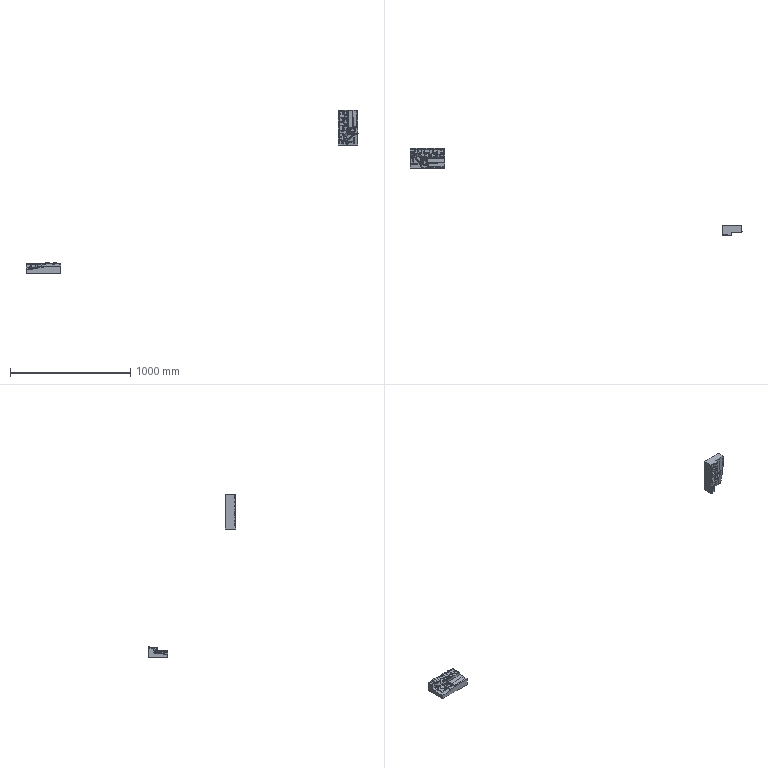NC program | NX | posted with a generic post | part box 2756 x 729.572 x 1353 mm
Lines 37177 to 38047 of 180527:
(STREAMLINE , TOOL : B6)
N74334 M6
N74336 G54
N74338 G17 G0 G90 X286.496 Y153.625 B0. C0. S3000 M3
N74340 G43 Z10. H0
N74342 Z-2.
N74344 G94 G1 Z-7.768 F2500.
N74346 X281.919
N74348 X279.629 Z-7.759
N74350 X277.339 Z-7.719
N74352 X268.2 Y153.624 Z-7.574
N74354 X265.889 Y153.623 Z-7.541
N74356 X263.472 Z-7.507
N74358 X262.453 Z-7.486
N74360 X261.884 Z-7.423
N74362 X261.325 Y153.622 Z-7.305
N74364 X260.778 Z-7.133
N74366 X260.25 Y153.621 Z-6.911
N74368 X259.746 Y153.62 Z-6.64
N74370 X259.271 Y153.619 Z-6.322
N74372 X258.828 Y153.618 Z-5.96
N74374 X258.416 Y153.617 Z-5.561
N74376 X258.01 Y153.616 Z-5.158
N74378 X257.578 Y153.615 Z-4.781
N74380 X257.114 Y153.614 Z-4.448
N74382 X256.619 Y153.613 Z-4.16
N74384 X256.098 Y153.612 Z-3.921
N74386 X255.558 Z-3.732
N74388 X255.002 Y153.611 Z-3.595
N74390 X254.438 Z-3.514
N74392 X253.292 Z-3.475
N74394 X251.002 Y153.61 Z-3.437
N74396 X241.841 Y153.609 Z-3.298
N74398 X232.68 Y153.608 Z-3.182
N74400 X230.389 Z-3.156
N74402 X228.099 Z-3.144
N74404 X227.53 Z-3.201
N74406 X226.969 Z-3.313
N74408 X226.42 Y153.609 Z-3.478
N74410 X225.89 Z-3.694
N74412 X225.382 Y153.61 Z-3.959
N74414 X224.904 Y153.611 Z-4.271
N74416 X224.458 Y153.612 Z-4.627
N74418 X224.041 Y153.613 Z-5.023
N74420 X223.21 Y153.615 Z-5.811
N74422 X222.756 Y153.616 Z-6.159
N74424 X222.271 Y153.617 Z-6.461
N74426 X221.756 Y153.618 Z-6.716
N74428 X221.222 Z-6.92
N74430 X220.671 Y153.619 Z-7.073
N74432 X220.107 Z-7.173
N74434 X219.537 Z-7.218
N74436 X218.964 Z-7.221
N74438 X217.847
N74440 X215.489 Z-7.225
N74442 X206.373 Y153.618 Z-7.252
N74444 X203.936 Z-7.261
N74446 X201.559 Z-7.271
N74448 X199.489 Z-7.282
N74450 X198.923 Z-7.285
N74452 X198.35 Z-7.266
N74454 X197.783 Y153.617 Z-7.192
N74456 X197.226 Z-7.063
N74458 X196.682 Y153.616 Z-6.881
N74460 X196.159 Z-6.65
N74462 X195.66 Y153.615 Z-6.369
N74464 X195.191 Y153.614 Z-6.042
N74466 X194.755 Y153.613 Z-5.672
N74468 X194.345 Y153.612 Z-5.27
N74470 X193.922 Y153.611 Z-4.886
N74472 X193.471 Y153.609 Z-4.532
N74474 X192.997 Y153.608 Z-4.212
N74476 X192.501 Z-3.927
N74478 X191.985 Y153.607 Z-3.678
N74480 X191.453 Y153.606 Z-3.466
N74482 X190.907 Z-3.293
N74484 X190.351 Y153.605 Z-3.16
N74486 X189.786 Z-3.066
N74488 X189.216 Z-3.013
N74490 X188.644 Z-3.001
N74492 X188.071 Z-3.011
N74494 X186.926 Z-3.032
N74496 X184.636 Z-3.074
N74498 X182.346 Z-3.118
N74500 X180.056 Z-3.163
N74502 X170.896 Y153.604 Z-3.361
N74504 X168.606 Z-3.414
N74506 X166.317 Z-3.469
N74508 X164.027 Z-3.526
N74510 X163.454 Z-3.545
N74512 X162.884 Y153.605 Z-3.598
N74514 X162.32 Z-3.693
N74516 X161.763 Z-3.827
N74518 X161.218 Y153.606 Z-4.002
N74520 X160.687 Z-4.215
N74522 X160.172 Y153.607 Z-4.464
N74524 X159.676 Y153.608 Z-4.751
N74526 X159.202 Y153.609 Z-5.072
N74528 X158.752 Y153.61 Z-5.426
N74530 X157.915 Y153.612 Z-6.207
N74532 X157.466 Y153.613 Z-6.563
N74534 X156.987 Y153.614 Z-6.873
N74536 X156.477 Z-7.138
N74538 X155.947 Y153.615 Z-7.352
N74540 X155.398 Z-7.516
N74542 X154.837 Y153.616 Z-7.626
N74544 X154.268 Z-7.681
N74546 X153.695 Z-7.691
N74548 X144.534 Y153.615 Z-7.737
N74550 X133.081 Z-7.773
N74552 X126.21 Y153.614 Z-7.781
N74554 X123.849 Z-7.782
N74556 X121.629
N74558 X121.342 Z-7.777
N74560 X121.058 Z-7.747
N74562 X120.778 Y153.613 Z-7.69
N74564 X120.504 Z-7.606
N74566 X120.24 Z-7.496
N74568 X119.987 Y153.612 Z-7.362
N74570 X119.497 Y153.611 Z-7.065
N74572 X118.999 Z-6.789
N74574 X118.485 Y153.61 Z-6.529
N74576 X117.966 Y153.609 Z-6.29
N74578 X117.437 Y153.608 Z-6.07
N74580 X116.9 Z-5.871
N74582 X116.356 Y153.607 Z-5.692
N74584 X115.806 Z-5.534
N74586 X115.249 Y153.606 Z-5.399
N74588 X114.683 Z-5.32
N74590 X114.11 Z-5.307
N74592 X112.966 Z-5.347
N74594 X108.388 Z-5.507
N74596 X99.231 Z-5.828
N74598 X96.942 Y153.607 Z-5.908
N74600 X95.798 Z-5.948
N74602 X95.225 Z-5.969
N74604 X94.656 Z-6.027
N74606 X94.098 Z-6.151
N74608 X93.557 Y153.608 Z-6.337
N74610 X92.53 Y153.609 Z-6.86
N74612 X91.543 Y153.611 Z-7.425
N74614 X90.999 Z-7.602
N74616 X90.433 Z-7.673
N74618 X81.268 Y153.61 Z-7.606
N74620 X72.108 Y153.609 Z-7.519
N74622 X70.964 Z-7.507
N74624 X70.397 Z-7.436
N74626 X69.853 Y153.608 Z-7.258
N74628 X67.878 Y153.605 Z-6.103
N74630 X66.843 Y153.603 Z-5.612
N74632 X65.775 Y153.602 Z-5.202
N74634 X64.677 Y153.601 Z-4.873
N74636 X63.559 Y153.6 Z-4.628
N74638 X62.425 Z-4.47
N74640 X61.282 Z-4.4
N74642 X47.54 Y153.598 Z-4.241
N74644 X46.395 Z-4.263
N74646 X45.256 Z-4.373
N74648 X44.132 Y153.599 Z-4.57
N74650 X43.018 Y153.6 Z-4.854
N74652 X41.934 Y153.601 Z-5.219
N74654 X40.88 Y153.602 Z-5.666
N74656 X39.861 Y153.603 Z-6.19
N74658 X38.879 Y153.605 Z-6.78
N74660 X38.351 Z-6.997
N74662 X37.79 Y153.606 Z-7.109
N74664 X36.645 Z-7.116
N74666 X0. Y153.605 Z-6.692
N74668 Z-6.832
N74670 X36.661 Y153.606 Z-7.256
N74672 X37.807 Z-7.25
N74674 X38.369 Y153.605 Z-7.14
N74676 X38.898 Z-6.925
N74678 X39.879 Y153.603 Z-6.334
N74680 X40.892 Y153.602 Z-5.8
N74682 X41.943 Y153.601 Z-5.347
N74684 X43.027 Y153.6 Z-4.979
N74686 X44.141 Y153.599 Z-4.697
N74688 X45.267 Y153.598 Z-4.506
N74690 X46.406 Z-4.401
N74692 X47.552 Z-4.381
N74694 X61.3 Y153.6 Z-4.54
N74696 X62.444 Z-4.608
N74698 X63.579 Z-4.762
N74700 X64.697 Y153.601 Z-5.007
N74702 X65.794 Y153.602 Z-5.341
N74704 X66.858 Y153.604 Z-5.759
N74706 X67.887 Y153.605 Z-6.261
N74708 X69.864 Y153.608 Z-7.408
N74710 X70.41 Y153.609 Z-7.579
N74712 X70.977 Z-7.647
N74714 X72.122 Z-7.659
N74716 X83.562 Y153.611 Z-7.764
N74718 X90.455 Z-7.813
N74720 X91.022 Z-7.745
N74722 X91.567 Y153.61 Z-7.571
N74724 X92.552 Y153.609 Z-7.003
N74726 X93.578 Y153.607 Z-6.478
N74728 X94.118 Z-6.289
N74730 X94.676 Z-6.163
N74732 X95.245 Z-6.1
N74734 X95.817 Z-6.076
N74736 X96.962 Z-6.035
N74738 X99.252 Y153.606 Z-5.954
N74740 X108.412 Z-5.633
N74742 X112.992 Z-5.473
N74744 X114.137 Z-5.436
N74746 X114.71 Z-5.454
N74748 X115.276 Z-5.535
N74750 X115.832 Y153.607 Z-5.672
N74752 X116.382 Z-5.833
N74754 X116.924 Y153.608 Z-6.016
N74756 X117.458 Z-6.221
N74758 X117.985 Y153.609 Z-6.446
N74760 X118.499 Y153.61 Z-6.691
N74762 X119.51 Y153.612 Z-7.232
N74764 X120.003 Z-7.52
N74766 X120.257 Y153.613 Z-7.648
N74768 X120.522 Z-7.753
N74770 X120.798 Z-7.833
N74772 X121.078 Y153.614 Z-7.888
N74774 X121.362 Z-7.917
N74776 X121.648 Z-7.922
N74778 X123.873 Z-7.921
N74780 X126.232
N74782 X137.689 Y153.615 Z-7.902
N74784 X144.564 Z-7.877
N74786 X153.729 Y153.616 Z-7.83
N74788 X154.303 Z-7.821
N74790 X154.872 Z-7.768
N74792 X155.434 Y153.615 Z-7.662
N74794 X155.984 Z-7.506
N74796 X156.516 Y153.614 Z-7.3
N74798 X157.029 Z-7.047
N74800 X157.512 Y153.613 Z-6.746
N74802 X157.963 Y153.612 Z-6.394
N74804 X158.797 Y153.609 Z-5.61
N74806 X159.243 Y153.608 Z-5.251
N74808 X159.713 Z-4.925
N74810 X160.205 Y153.607 Z-4.634
N74812 X160.717 Y153.606 Z-4.379
N74814 X161.246 Z-4.161
N74816 X161.79 Y153.605 Z-3.982
N74818 X162.345 Z-3.843
N74820 X162.908 Z-3.744
N74822 X163.478 Y153.604 Z-3.686
N74824 X164.05 Z-3.663
N74826 X166.341 Z-3.604
N74828 X168.631 Z-3.549
N74830 X170.922 Z-3.496
N74832 X180.086 Y153.605 Z-3.298
N74834 X182.377 Z-3.252
N74836 X184.668 Z-3.209
N74838 X186.959 Z-3.167
N74840 X188.104 Z-3.154
N74842 X188.676 Z-3.151
N74844 X189.247 Z-3.17
N74846 X189.816 Z-3.231
N74848 X190.378 Z-3.333
N74850 X190.931 Y153.606 Z-3.474
N74852 X191.473 Z-3.655
N74854 X192. Y153.607 Z-3.875
N74856 X192.51 Y153.608 Z-4.131
N74858 X193. Z-4.424
N74860 X193.468 Y153.609 Z-4.751
N74862 X195.199 Y153.614 Z-6.236
N74864 X195.673 Y153.615 Z-6.549
N74866 X196.176 Y153.616 Z-6.817
N74868 X196.701 Y153.617 Z-7.039
N74870 X197.247 Z-7.213
N74872 X197.805 Z-7.336
N74874 X198.372 Y153.618 Z-7.406
N74876 X198.945 Z-7.425
N74878 X199.511 Z-7.422
N74880 X201.592 Z-7.411
N74882 X203.966 Z-7.4
N74884 X206.398 Z-7.391
N74886 X215.521 Y153.619 Z-7.365
N74888 X217.877 Z-7.361
N74890 X218.995
N74892 X219.568 Z-7.358
N74894 X220.139 Z-7.315
N74896 X220.703 Z-7.22
N74898 X221.256 Y153.618 Z-7.073
N74900 X221.792 Z-6.877
N74902 X222.309 Y153.617 Z-6.633
N74904 X222.798 Y153.616 Z-6.341
N74906 X223.255 Y153.615 Z-5.999
N74908 X223.677 Y153.614 Z-5.611
N74910 X224.083 Y153.613 Z-5.208
N74912 X224.495 Y153.612 Z-4.808
N74914 X224.937 Y153.611 Z-4.446
N74916 X225.41 Y153.61 Z-4.129
N74918 X225.914 Y153.609 Z-3.858
N74920 X226.44 Z-3.635
N74922 X226.986 Y153.608 Z-3.463
N74924 X227.544 Z-3.344
N74926 X228.111 Z-3.278
N74928 X230.399 Z-3.266
N74930 X232.69 Z-3.289
N74932 X241.856 Y153.609 Z-3.399
N74934 X251.02 Y153.61 Z-3.532
N74936 X253.309 Y153.611 Z-3.589
N74938 X254.45 Z-3.648
N74940 X255.012 Z-3.74
N74942 X255.563 Y153.612 Z-3.885
N74944 X256.098 Z-4.083
N74946 X256.614 Y153.613 Z-4.331
N74948 X257.103 Y153.614 Z-4.625
N74950 X257.561 Y153.615 Z-4.965
N74952 X257.985 Y153.616 Z-5.347
N74954 X258.388 Y153.617 Z-5.754
N74956 X258.802 Y153.618 Z-6.151
N74958 X259.248 Y153.619 Z-6.507
N74960 X259.727 Y153.62 Z-6.814
N74962 X260.235 Y153.621 Z-7.074
N74964 X260.764 Y153.622 Z-7.287
N74966 X261.313 Z-7.452
N74968 X261.873 Y153.623 Z-7.565
N74970 X262.442 Z-7.626
N74972 X263.467 Z-7.647
N74974 X265.879 Z-7.681
N74976 X268.191 Y153.624 Z-7.714
N74978 X277.335 Y153.625 Z-7.859
N74980 X279.626 Z-7.899
N74982 X281.917 Z-7.907
N74984 X286.496
N74986 Z-8.047
N74988 X281.915
N74990 X279.623 Z-8.039
N74992 X277.331 Z-7.999
N74994 X268.182 Y153.624 Z-7.854
N74996 X265.87 Y153.623 Z-7.82
N74998 X263.463 Z-7.787
N75000 X262.432 Z-7.766
N75002 X261.862 Z-7.708
N75004 X261.301 Y153.622 Z-7.599
N75006 X260.751 Z-7.441
N75008 X260.219 Y153.621 Z-7.237
N75010 X259.709 Y153.62 Z-6.989
N75012 X259.225 Y153.619 Z-6.692
N75014 X258.775 Y153.618 Z-6.342
N75016 X258.36 Y153.617 Z-5.946
N75018 X257.961 Y153.616 Z-5.536
N75020 X257.543 Y153.615 Z-5.148
N75022 X257.091 Y153.614 Z-4.802
N75024 X256.608 Y153.613 Z-4.501
N75026 X256.098 Y153.612 Z-4.245
N75028 X255.568 Z-4.039
N75030 X255.021 Y153.611 Z-3.884
N75032 X254.463 Z-3.782
N75034 X253.895 Z-3.732
N75036 X253.326 Z-3.703
N75038 X251.039 Y153.61 Z-3.628
N75040 X241.87 Y153.609 Z-3.5
N75042 X232.701 Y153.608 Z-3.396
N75044 X230.409 Z-3.375
N75046 X229.264 Z-3.38
N75048 X228.123 Z-3.412
N75050 X227.558 Z-3.486
N75052 X227.003 Z-3.613
N75054 X226.46 Y153.609 Z-3.793
N75056 X225.938 Z-4.022
N75058 X225.438 Y153.61 Z-4.3
N75060 X224.969 Y153.611 Z-4.622
N75062 X224.532 Y153.612 Z-4.988
N75064 X224.126 Y153.613 Z-5.393
N75066 X223.723 Y153.614 Z-5.799
N75068 X223.301 Y153.615 Z-6.186
N75070 X222.839 Y153.616 Z-6.524
N75072 X222.347 Y153.617 Z-6.805
N75074 X221.827 Y153.618 Z-7.038
N75076 X221.289 Z-7.226
N75078 X220.735 Y153.619 Z-7.366
N75080 X220.171 Z-7.457
N75082 X219.6 Z-7.498
N75084 X219.026 Z-7.5
N75086 X217.906 Z-7.501
N75088 X215.552 Z-7.505
N75090 X206.424 Y153.618 Z-7.531
N75092 X203.997 Z-7.54
N75094 X201.626 Z-7.55
N75096 X199.534 Z-7.561
N75098 X198.967 Z-7.565
N75100 X198.394 Z-7.547
N75102 X197.826 Y153.617 Z-7.48
N75104 X197.268 Z-7.363
N75106 X196.72 Z-7.196
N75108 X196.193 Y153.616 Z-6.985
N75110 X195.687 Y153.615 Z-6.728
N75112 X195.208 Y153.614 Z-6.43
N75114 X193.465 Y153.609 Z-4.971
N75116 X193.004 Z-4.637
N75118 X192.52 Y153.608 Z-4.336
N75120 X192.015 Y153.607 Z-4.072
N75122 X191.493 Y153.606 Z-3.844
N75124 X190.955 Z-3.655
N75126 X190.405 Y153.605 Z-3.506
N75128 X189.845 Z-3.396
N75130 X189.279 Z-3.328
N75132 X188.709 Z-3.301
N75134 X188.137 Z-3.297
N75136 X186.993 Z-3.302
N75138 X184.7 Z-3.343
N75140 X182.408 Z-3.387
N75142 X180.116 Z-3.433
N75144 X170.948 Y153.604 Z-3.63
N75146 X168.656 Z-3.684
N75148 X166.365 Z-3.739
N75150 X164.073 Z-3.8
N75152 X163.501 Z-3.827
N75154 X162.932 Y153.605 Z-3.889
N75156 X162.37 Z-3.993
N75158 X161.816 Z-4.137
N75160 X161.275 Y153.606 Z-4.321
N75162 X160.748 Z-4.544
N75164 X160.239 Y153.607 Z-4.804
N75166 X159.75 Y153.608 Z-5.1
N75168 X159.284 Z-5.431
N75170 X158.843 Y153.609 Z-5.795
N75172 X158.012 Y153.612 Z-6.582
N75174 X157.558 Y153.613 Z-6.929
N75176 X157.071 Z-7.22
N75178 X156.555 Y153.614 Z-7.462
N75180 X156.021 Y153.615 Z-7.659
N75182 X155.47 Z-7.809
N75184 X154.907 Y153.616 Z-7.91
N75186 X154.337 Z-7.961
N75188 X153.763 Z-7.97
N75190 X144.594 Y153.615 Z-8.017
N75192 X133.131 Z-8.052
N75194 X126.254 Y153.614 Z-8.06
N75196 X123.897 Z-8.061
N75198 X121.668 Z-8.062
N75200 X121.382 Z-8.057
N75202 X121.097 Z-8.029
N75204 X120.817 Y153.613 Z-7.977
N75206 X120.541 Z-7.9
N75208 X120.274 Z-7.8
N75210 X120.019 Y153.612 Z-7.677
N75212 X119.522 Z-7.398
N75214 X118.514 Y153.61 Z-6.854
N75216 X118.003 Y153.609 Z-6.603
N75218 X117.48 Z-6.371
N75220 X116.948 Y153.608 Z-6.162
N75222 X116.407 Y153.607 Z-5.975
N75224 X115.858 Z-5.811
N75226 X115.303 Y153.606 Z-5.671
N75228 X114.737 Z-5.587
N75230 X114.165 Z-5.566
N75232 X113.019 Z-5.599
N75234 X108.437 Z-5.76
N75236 X99.273 Z-6.081
N75238 X96.982 Y153.607 Z-6.161
N75240 X95.836 Z-6.204
N75242 X95.264 Z-6.231
N75244 X94.696 Z-6.298
N75246 X94.139 Z-6.427
N75248 X93.599 Z-6.618
N75250 X93.082 Y153.608 Z-6.866
N75252 X92.575 Y153.609 Z-7.147
N75254 X92.09 Y153.61 Z-7.444
N75256 X91.847 Z-7.592
N75258 X91.59 Z-7.717
N75260 X91.322 Y153.611 Z-7.816
N75262 X91.044 Z-7.888
N75264 X90.762 Z-7.933
N75266 X90.477 Z-7.953
N75268 X81.304 Y153.61 Z-7.885
N75270 X72.136 Y153.609 Z-7.799
N75272 X70.99 Z-7.787
N75274 X70.423 Z-7.722
N75276 X69.875 Z-7.558
N75278 X67.895 Y153.605 Z-6.419
N75280 X66.873 Y153.604 Z-5.906
N75282 X65.812 Y153.602 Z-5.479
N75284 X64.717 Y153.601 Z-5.141
N75286 X63.598 Y153.6 Z-4.895
N75288 X62.463 Z-4.745
N75290 X61.318 Z-4.68
N75292 X47.564 Y153.598 Z-4.521
N75294 X46.418 Z-4.54
N75296 X45.278 Z-4.639
N75298 X44.15 Y153.599 Z-4.824
N75300 X43.036 Y153.6 Z-5.105
N75302 X41.952 Y153.601 Z-5.475
N75304 X40.904 Y153.602 Z-5.934
N75306 X38.916 Y153.605 Z-7.071
N75308 X38.386 Z-7.283
N75310 X37.824 Y153.606 Z-7.391
N75312 X36.678 Z-7.396
N75314 X0. Y153.605 Z-6.972
N75316 Z-7.112
N75318 X36.694 Y153.606 Z-7.535
N75320 X37.841 Z-7.532
N75322 X38.403 Y153.605 Z-7.426
N75324 X38.935 Z-7.216
N75326 X40.916 Y153.602 Z-6.069
N75328 X41.961 Y153.601 Z-5.603
N75330 X43.045 Y153.6 Z-5.23
N75332 X44.16 Y153.599 Z-4.951
N75334 X45.289 Y153.598 Z-4.772
N75336 X46.429 Z-4.678
N75338 X47.576 Z-4.66
N75340 X61.337 Y153.6 Z-4.82
N75342 X62.481 Z-4.883
N75344 X63.618 Z-5.029
N75346 X64.737 Y153.601 Z-5.275
N75348 X65.831 Y153.602 Z-5.618
N75350 X66.889 Y153.604 Z-6.053
N75352 X67.903 Y153.605 Z-6.578
N75354 X69.887 Y153.609 Z-7.708
N75356 X70.436 Z-7.864
N75358 X71.004 Z-7.927
N75360 X72.15 Z-7.939
N75362 X83.602 Y153.611 Z-8.044
N75364 X90.499 Z-8.093
N75366 X90.784 Z-8.074
N75368 X91.067 Z-8.031
N75370 X91.345 Z-7.961
N75372 X91.614 Y153.61 Z-7.863
N75374 X91.871 Z-7.739
N75376 X92.114 Z-7.591
N75378 X92.598 Y153.609 Z-7.291
N75380 X93.104 Y153.608 Z-7.008
N75382 X93.62 Y153.607 Z-6.758
N75384 X94.159 Z-6.565
N75386 X94.715 Z-6.433
N75388 X95.284 Z-6.363
N75390 X95.855 Z-6.332
N75392 X97.001 Z-6.288
N75394 X99.293 Y153.606 Z-6.207
N75396 X108.462 Z-5.886
N75398 X110.754 Z-5.805
N75400 X113.046 Z-5.725
N75402 X114.192 Z-5.696
N75404 X114.764 Z-5.72
N75406 X115.329 Z-5.808
N75408 X115.885 Y153.607 Z-5.949
N75410 X116.433 Z-6.117
N75412 X116.972 Y153.608 Z-6.308
N75414 X117.502 Y153.609 Z-6.522
N75416 X118.022 Z-6.759
N75418 X118.529 Y153.61 Z-7.017
N75420 X119.535 Y153.612 Z-7.565
N75422 X120.034 Z-7.835
N75424 X120.292 Y153.613 Z-7.952
N75426 X120.559 Z-8.047
N75428 X120.836 Z-8.121
N75430 X121.117 Y153.614 Z-8.17
N75432 X121.402 Z-8.197
N75434 X121.688 Z-8.201
N75436 X123.921
N75438 X126.276 Z-8.2
N75440 X137.743 Y153.615 Z-8.181
N75442 X144.624 Z-8.156
N75444 X153.798 Y153.616 Z-8.109
N75446 X154.372 Z-8.101
N75448 X154.942 Z-8.052
N75450 X155.505 Y153.615 Z-7.955
N75452 X156.058 Z-7.812
N75454 X156.594 Y153.614 Z-7.624
N75456 X157.112 Y153.613 Z-7.393
N75458 X157.603 Y153.612 Z-7.111
N75460 X158.061 Y153.611 Z-6.769
N75462 X158.889 Y153.609 Z-5.979
N75464 X159.325 Y153.608 Z-5.611
N75466 X159.787 Y153.607 Z-5.275
N75468 X160.272 Z-4.974
N75470 X160.779 Y153.606 Z-4.709
N75472 X161.303 Z-4.481
N75474 X161.842 Y153.605 Z-4.292
N75476 X162.395 Z-4.144
N75478 X162.956 Z-4.035
N75480 X163.525 Y153.604 Z-3.968
N75482 X164.096 Z-3.937
N75484 X166.389 Z-3.873
N75486 X168.681 Z-3.818
N75488 X170.974 Z-3.765
N75490 X180.146 Y153.605 Z-3.567
N75492 X182.439 Z-3.522
N75494 X184.732 Z-3.478
N75496 X187.026 Z-3.438
N75498 X188.17 Z-3.44
N75500 X188.741 Z-3.45
N75502 X189.31 Z-3.485
N75504 X189.875 Z-3.561
N75506 X190.432 Z-3.679
N75508 X190.979 Y153.606 Z-3.836
N75510 X191.513 Z-4.033
N75512 X192.031 Y153.607 Z-4.269
N75514 X192.53 Y153.608 Z-4.541
N75516 X193.007 Y153.609 Z-4.849
N75518 X193.462 Z-5.19
N75520 X194.335 Y153.612 Z-5.928
N75522 X194.763 Y153.613 Z-6.298
N75524 X195.217 Y153.614 Z-6.623
N75526 X195.7 Y153.615 Z-6.908
N75528 X196.209 Y153.616 Z-7.152
N75530 X196.739 Y153.617 Z-7.354
N75532 X197.288 Z-7.512
N75534 X197.848 Y153.618 Z-7.624
N75536 X198.416 Z-7.688
N75538 X198.99 Z-7.705
N75540 X199.557 Z-7.701
N75542 X201.659 Z-7.69
N75544 X204.027 Z-7.68
N75546 X206.449 Z-7.671
N75548 X215.583 Y153.619 Z-7.645
N75550 X217.936 Z-7.641
N75552 X220.202 Z-7.599
N75554 X221.323 Y153.618 Z-7.378
N75556 X222.385 Y153.617 Z-6.977
N75558 X222.881 Y153.616 Z-6.706
N75560 X223.346 Y153.615 Z-6.373
N75562 X224.168 Y153.613 Z-5.577
N75564 X225.002 Y153.611 Z-4.798
N75566 X225.962 Y153.609 Z-4.186
N75568 X227.02 Y153.608 Z-3.763
N75570 X228.135 Z-3.546
N75572 X230.418 Z-3.485
N75574 X232.712 Z-3.503
N75576 X241.885 Y153.609 Z-3.601
N75578 X251.058 Y153.61 Z-3.723
N75580 X252.203 Y153.611 Z-3.758
N75582 X253.344 Z-3.818
N75584 X253.911 Z-3.856
N75586 X254.475 Z-3.916
N75588 X255.03 Z-4.028
N75590 X255.573 Y153.612 Z-4.192
N75592 X256.099 Z-4.408
N75594 X256.603 Y153.613 Z-4.671
N75596 X257.08 Y153.614 Z-4.979
N75598 X257.525 Y153.615 Z-5.332
N75600 X257.937 Y153.616 Z-5.726
N75602 X258.332 Y153.617 Z-6.138
N75604 X258.749 Y153.618 Z-6.533
N75606 X259.202 Y153.619 Z-6.877
N75608 X259.69 Y153.62 Z-7.163
N75610 X260.204 Y153.621 Z-7.401
N75612 X260.738 Y153.622 Z-7.595
N75614 X261.289 Z-7.746
N75616 X261.85 Y153.623 Z-7.85
N75618 X262.421 Z-7.906
N75620 X263.458 Z-7.927
N75622 X265.861 Z-7.96
N75624 X268.173 Y153.624 Z-7.993
N75626 X277.326 Y153.625 Z-8.138
N75628 X279.62 Z-8.178
N75630 X281.913 Z-8.187
N75632 X286.496
N75634 Z-8.326
N75636 X281.911
N75638 X279.617 Z-8.318
N75640 X277.322 Z-8.278
N75642 X268.163 Y153.624 Z-8.133
N75644 X265.852 Y153.623 Z-8.1
N75646 X263.453 Z-8.067
N75648 X262.41 Z-8.047
N75650 X261.839 Z-7.993
N75652 X261.277 Y153.622 Z-7.894
N75654 X260.725 Z-7.75
N75656 X260.189 Y153.621 Z-7.564
N75658 X259.672 Y153.62 Z-7.337
N75660 X259.18 Y153.619 Z-7.063
N75662 X258.722 Y153.618 Z-6.724
N75664 X258.305 Y153.617 Z-6.331
N75666 X257.912 Y153.616 Z-5.915
N75668 X257.507 Y153.615 Z-5.516
N75670 X257.068 Y153.614 Z-5.157
N75672 X256.597 Y153.613 Z-4.841
N75674 X256.099 Y153.612 Z-4.57
N75676 X255.578 Z-4.346
N75678 X255.039 Y153.611 Z-4.172
N75680 X254.488 Z-4.05
N75682 X253.926 Z-3.979
N75684 X253.361 Z-3.932
N75686 X252.222 Z-3.859
N75688 X251.077 Y153.61 Z-3.819
N75690 X241.9 Y153.609 Z-3.703
N75692 X232.722 Y153.608 Z-3.61
N75694 X230.428 Z-3.594
N75696 X229.284 Z-3.616
N75698 X228.147 Z-3.68
N75700 X227.586 Z-3.771
N75702 X227.036 Z-3.913
N75704 X226.501 Y153.609 Z-4.107
N75706 X225.986 Z-4.35
N75708 X225.494 Y153.61 Z-4.64
N75710 X225.034 Y153.611 Z-4.973
N75712 X224.607 Y153.612 Z-5.349
N75714 X224.21 Y153.613 Z-5.762
N75716 X223.815 Y153.614 Z-6.176
N75718 X223.391 Y153.615 Z-6.561
N75720 X222.923 Y153.616 Z-6.888
N75722 X222.423 Y153.617 Z-7.15
N75724 X221.898 Y153.618 Z-7.361
N75726 X221.356 Z-7.531
N75728 X220.8 Y153.619 Z-7.658
N75730 X220.234 Z-7.741
N75732 X219.662 Z-7.778
N75734 X219.089 Z-7.78
N75736 X217.965 Z-7.781
N75738 X215.614 Z-7.784
N75740 X206.474 Y153.618 Z-7.81
N75742 X204.058 Z-7.819
N75744 X201.692 Z-7.83
N75746 X199.58 Z-7.841
N75748 X198.438 Z-7.829
N75750 X197.869 Z-7.768
N75752 X197.309 Y153.617 Z-7.662
N75754 X196.758 Z-7.511
N75756 X196.226 Y153.616 Z-7.32
N75758 X195.713 Y153.615 Z-7.087
N75760 X195.226 Y153.614 Z-6.817
N75762 X194.766 Y153.613 Z-6.507
N75764 X194.331 Y153.612 Z-6.147
N75766 X193.458 Y153.609 Z-5.409
N75768 X193.011 Z-5.061
N75770 X192.539 Y153.608 Z-4.745
N75772 X192.046 Y153.607 Z-4.466
N75774 X191.533 Y153.606 Z-4.223
N75776 X191.003 Z-4.018
N75778 X190.459 Y153.605 Z-3.852
N75780 X189.904 Z-3.727
N75782 X189.342 Z-3.642
N75784 X188.774 Z-3.6
N75786 X188.204 Z-3.583
N75788 X187.059 Z-3.573
N75790 X184.765 Z-3.613
N75792 X182.471 Z-3.657
N75794 X180.176 Z-3.702
N75796 X171. Y153.604 Z-3.9
N75798 X168.707 Z-3.953
N75800 X166.413 Z-4.008
N75802 X164.119 Z-4.074
N75804 X163.548 Z-4.109
N75806 X162.98 Y153.605 Z-4.18
N75808 X162.42 Z-4.294
N75810 X161.869 Z-4.447
N75812 X161.331 Z-4.641
N75814 X160.809 Y153.606 Z-4.873
N75816 X160.306 Y153.607 Z-5.143
N75818 X159.823 Z-5.45
N75820 X159.366 Y153.608 Z-5.79
N75822 X158.934 Y153.609 Z-6.163
N75824 X158.11 Y153.611 Z-6.957
N75826 X157.649 Y153.612 Z-7.294
N75828 X157.154 Y153.613 Z-7.566
N75830 X156.633 Y153.614 Z-7.786
N75832 X156.095 Y153.615 Z-7.965
N75834 X155.541 Z-8.102
N75836 X154.977 Y153.616 Z-8.194
N75838 X154.406 Z-8.24
N75840 X153.832 Z-8.249
N75842 X144.654 Y153.615 Z-8.296
N75844 X133.181 Z-8.332
N75846 X126.298 Y153.614 Z-8.34
N75848 X123.945 Z-8.341
N75850 X121.708
N75852 X121.422 Z-8.337
N75854 X121.137 Z-8.312
N75856 X120.855 Y153.613 Z-8.264
N75858 X120.578 Z-8.194
N75860 X120.309 Z-8.104
N75862 X120.05 Y153.612 Z-7.992
N75864 X119.547 Z-7.731
N75866 X118.544 Y153.61 Z-7.18
N75868 X118.041 Y153.609 Z-6.915
N75870 X117.524 Z-6.673
N75872 X116.996 Y153.608 Z-6.453
N75874 X116.459 Y153.607 Z-6.258
N75876 X115.911 Z-6.087
N75878 X115.356 Y153.606 Z-5.944
N75880 X114.791 Z-5.854
N75882 X114.219 Z-5.826
N75884 X113.073 Z-5.851
N75886 X110.78 Z-5.932
N75888 X108.487 Z-6.012
N75890 X99.314 Z-6.334
N75892 X97.021 Y153.607 Z-6.414
N75894 X95.875 Z-6.46
N75896 X95.303 Z-6.494
N75898 X94.735 Z-6.568
N75900 X94.179 Z-6.703
N75902 X93.641 Z-6.899
N75904 X93.125 Y153.608 Z-7.15
N75906 X92.621 Y153.609 Z-7.435
N75908 X92.138 Y153.61 Z-7.737
N75910 X91.895 Z-7.885
N75912 X91.637 Z-8.009
N75914 X91.368 Y153.611 Z-8.106
N75916 X91.089 Z-8.174
N75918 X90.806 Z-8.215
N75920 X90.521 Z-8.233
N75922 X81.34 Y153.61 Z-8.165
N75924 X72.163 Y153.609 Z-8.079
N75926 X71.017 Z-8.067
N75928 X70.448 Z-8.007
N75930 X69.898 Z-7.858
N75932 X67.911 Y153.605 Z-6.736
N75934 X66.904 Y153.604 Z-6.2
N75936 X65.85 Y153.602 Z-5.757
N75938 X64.757 Y153.601 Z-5.41
N75940 X63.638 Y153.6 Z-5.163
N75942 X62.5 Z-5.02
N75944 X61.355 Z-4.96
N75946 X47.588 Y153.598 Z-4.8
N75948 X46.441 Z-4.816
N75950 X45.299 Z-4.905
N75952 X44.169 Y153.599 Z-5.078
N75954 X43.054 Y153.6 Z-5.355
N75956 X41.97 Y153.601 Z-5.731
N75958 X40.927 Y153.602 Z-6.203
N75960 X38.953 Y153.605 Z-7.362
N75962 X38.421 Z-7.569
N75964 X37.857 Y153.606 Z-7.672
N75966 X36.71 Z-7.675
N75968 X0. Y153.605 Z-7.251
N75970 Z-7.391
N75972 X36.727 Y153.606 Z-7.815
N75974 X37.874 Z-7.813
N75976 X38.438 Y153.605 Z-7.713
N75978 X38.972 Z-7.507
N75980 X40.939 Y153.602 Z-6.337
N75982 X41.979 Y153.601 Z-5.859
N75984 X43.062 Y153.6 Z-5.481
N75986 X44.179 Y153.599 Z-5.206
N75988 X45.31 Y153.598 Z-5.038
N75990 X46.452 Z-4.955
N75992 X47.6 Z-4.94
N75994 X61.373 Y153.6 Z-5.1
N75996 X62.519 Z-5.158
N75998 X63.657 Z-5.297
N76000 X64.777 Y153.601 Z-5.544
N76002 X65.869 Y153.602 Z-5.896
N76004 X66.919 Y153.604 Z-6.347
N76006 X67.92 Y153.605 Z-6.895
N76008 X68.901 Y153.607 Z-7.484
N76010 X69.909 Y153.609 Z-8.008
N76012 X70.461 Z-8.15
N76014 X71.03 Z-8.207
N76016 X72.177 Z-8.219
N76018 X83.641 Y153.611 Z-8.324
N76020 X90.542 Z-8.373
N76022 X90.828 Z-8.356
N76024 X91.111 Z-8.317
N76026 X91.391 Z-8.251
N76028 X91.661 Y153.61 Z-8.155
N76030 X91.919 Z-8.032
N76032 X92.162 Z-7.884
N76034 X92.643 Y153.609 Z-7.579
N76036 X93.147 Y153.608 Z-7.292
N76038 X93.662 Y153.607 Z-7.039
N76040 X94.2 Z-6.842
N76042 X94.755 Z-6.703
N76044 X95.322 Z-6.626
N76046 X95.894 Z-6.588
N76048 X97.041 Z-6.54
N76050 X99.335 Y153.606 Z-6.46
N76052 X108.511 Z-6.138
N76054 X110.805 Z-6.058
N76056 X113.1 Z-5.977
N76058 X114.247 Z-5.956
N76060 X114.818 Z-5.987
N76062 X115.383 Z-6.08
N76064 X115.938 Y153.607 Z-6.226
N76066 X116.484 Z-6.4
N76068 X117.02 Y153.608 Z-6.599